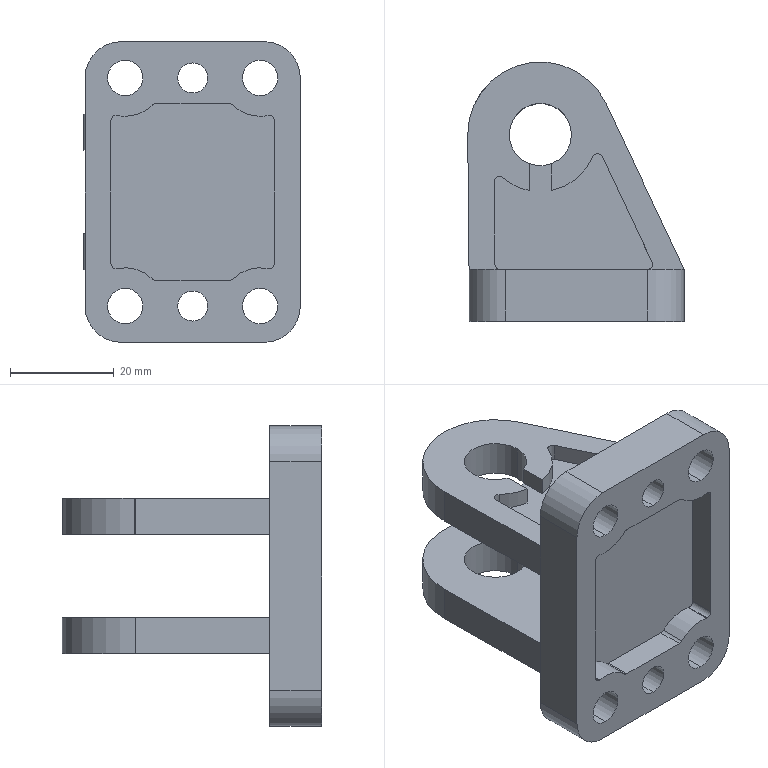Part | SolidWorks | features ICE 9, Fillet 2, HoleWzd 2, RevCut 2, Draft 1, Extrusion 1 | 1 solid | 84 faces | box 41.75 x 50 x 58 mm | volume 28986 mm3 | cylinder 53 | plane 31 | commonest cylinder face diameters 2 x20 6.8 x8 14.8 x6 5.8 x4 12 x4 14 x4